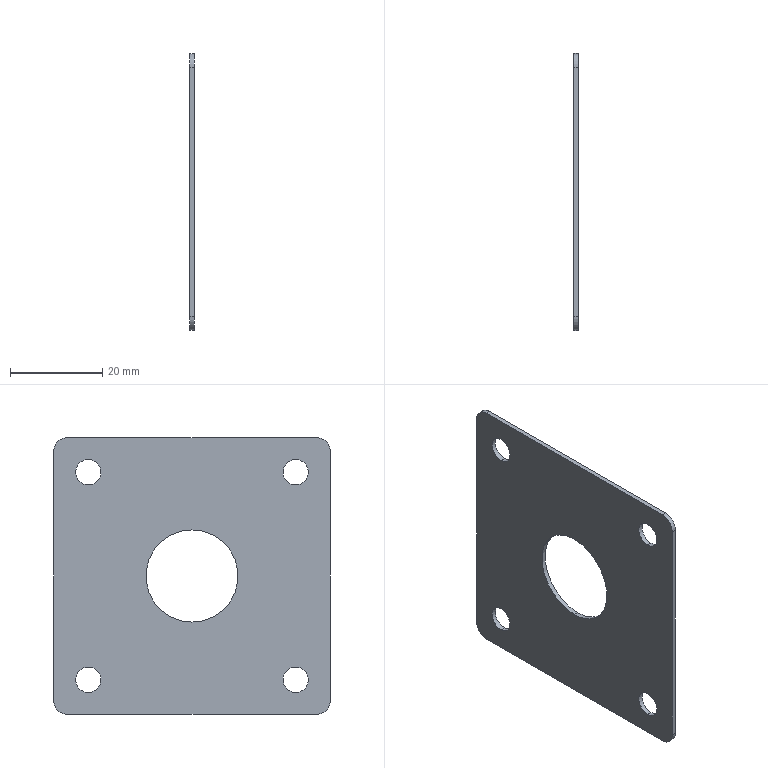Part | STEP file | FFH80-GY-022^FFH85-PL-M75-B3-01_three-axis module | 1 solid | 20 faces | box 1 x 60 x 60 mm | volume 3183 mm3 | cylinder 14 | plane 6 | commonest cylinder face diameters 5.5 x8 6 x4 20 x2
STEP:
#1=CARTESIAN_POINT('',(0.,22.5,-19.75));
#2=VERTEX_POINT('',#1);
#3=CARTESIAN_POINT('',(0.,22.5,-25.25));
#4=VERTEX_POINT('',#3);
#5=CARTESIAN_POINT('',(0.,22.5,-22.5));
#6=DIRECTION('',(1.,0.,0.));
#7=DIRECTION('',(0.,0.,-1.));
#8=AXIS2_PLACEMENT_3D('',#5,#6,#7);
#9=CIRCLE('',#8,2.75);
#10=EDGE_CURVE('',#2,#4,#9,.T.);
#11=ORIENTED_EDGE('',*,*,#10,.F.);
#12=CARTESIAN_POINT('',(1.,22.5,-19.75));
#13=VERTEX_POINT('',#12);
#14=CARTESIAN_POINT('',(1.,22.5,-19.75));
#15=DIRECTION('',(1.,0.,0.));
#16=VECTOR('',#15,1000.);
#17=LINE('',#14,#16);
#18=EDGE_CURVE('',#2,#13,#17,.T.);
#19=ORIENTED_EDGE('',*,*,#18,.T.);
#20=CARTESIAN_POINT('',(1.,22.5,-25.25));
#21=VERTEX_POINT('',#20);
#22=CARTESIAN_POINT('',(1.,22.5,-22.5));
#23=DIRECTION('',(1.,0.,0.));
#24=DIRECTION('',(0.,0.,-1.));
#25=AXIS2_PLACEMENT_3D('',#22,#23,#24);
#26=CIRCLE('',#25,2.75);
#27=EDGE_CURVE('',#13,#21,#26,.T.);
#28=ORIENTED_EDGE('',*,*,#27,.T.);
#29=CARTESIAN_POINT('',(1.,22.5,-25.25));
#30=DIRECTION('',(1.,0.,0.));
#31=VECTOR('',#30,1000.);
#32=LINE('',#29,#31);
#33=EDGE_CURVE('',#4,#21,#32,.T.);
#34=ORIENTED_EDGE('',*,*,#33,.F.);
#35=EDGE_LOOP('',(#11,#19,#28,#34));
#36=FACE_OUTER_BOUND('',#35,.T.);
#37=CARTESIAN_POINT('',(1.,22.5,-22.5));
#38=DIRECTION('',(1.,0.,0.));
#39=DIRECTION('',(0.,0.,-1.));
#40=AXIS2_PLACEMENT_3D('',#37,#38,#39);
#41=CYLINDRICAL_SURFACE('',#40,2.75);
#42=ADVANCED_FACE('',(#36),#41,.F.);
#43=CARTESIAN_POINT('',(0.,22.5,25.25));
#44=VERTEX_POINT('',#43);
#45=CARTESIAN_POINT('',(0.,22.5,19.75));
#46=VERTEX_POINT('',#45);
#47=CARTESIAN_POINT('',(0.,22.5,22.5));
#48=DIRECTION('',(1.,0.,0.));
#49=DIRECTION('',(0.,0.,-1.));
#50=AXIS2_PLACEMENT_3D('',#47,#48,#49);
#51=CIRCLE('',#50,2.75);
#52=EDGE_CURVE('',#44,#46,#51,.T.);
#53=ORIENTED_EDGE('',*,*,#52,.F.);
#54=CARTESIAN_POINT('',(1.,22.5,25.25));
#55=VERTEX_POINT('',#54);
#56=CARTESIAN_POINT('',(1.,22.5,25.25));
#57=DIRECTION('',(1.,0.,0.));
#58=VECTOR('',#57,1000.);
#59=LINE('',#56,#58);
#60=EDGE_CURVE('',#44,#55,#59,.T.);
#61=ORIENTED_EDGE('',*,*,#60,.T.);
#62=CARTESIAN_POINT('',(1.,22.5,19.75));
#63=VERTEX_POINT('',#62);
#64=CARTESIAN_POINT('',(1.,22.5,22.5));
#65=DIRECTION('',(1.,0.,0.));
#66=DIRECTION('',(0.,0.,-1.));
#67=AXIS2_PLACEMENT_3D('',#64,#65,#66);
#68=CIRCLE('',#67,2.75);
#69=EDGE_CURVE('',#55,#63,#68,.T.);
#70=ORIENTED_EDGE('',*,*,#69,.T.);
#71=CARTESIAN_POINT('',(1.,22.5,19.75));
#72=DIRECTION('',(1.,0.,0.));
#73=VECTOR('',#72,1000.);
#74=LINE('',#71,#73);
#75=EDGE_CURVE('',#46,#63,#74,.T.);
#76=ORIENTED_EDGE('',*,*,#75,.F.);
#77=EDGE_LOOP('',(#53,#61,#70,#76));
#78=FACE_OUTER_BOUND('',#77,.T.);
#79=CARTESIAN_POINT('',(1.,22.5,22.5));
#80=DIRECTION('',(1.,0.,0.));
#81=DIRECTION('',(0.,0.,-1.));
#82=AXIS2_PLACEMENT_3D('',#79,#80,#81);
#83=CYLINDRICAL_SURFACE('',#82,2.75);
#84=ADVANCED_FACE('',(#78),#83,.F.);
#85=CARTESIAN_POINT('',(0.,-22.5,-19.75));
#86=VERTEX_POINT('',#85);
#87=CARTESIAN_POINT('',(0.,-22.5,-25.25));
#88=VERTEX_POINT('',#87);
#89=CARTESIAN_POINT('',(0.,-22.5,-22.5));
#90=DIRECTION('',(1.,0.,0.));
#91=DIRECTION('',(0.,0.,-1.));
#92=AXIS2_PLACEMENT_3D('',#89,#90,#91);
#93=CIRCLE('',#92,2.75);
#94=EDGE_CURVE('',#86,#88,#93,.T.);
#95=ORIENTED_EDGE('',*,*,#94,.F.);
#96=CARTESIAN_POINT('',(1.,-22.5,-19.75));
#97=VERTEX_POINT('',#96);
#98=CARTESIAN_POINT('',(1.,-22.5,-19.75));
#99=DIRECTION('',(1.,0.,0.));
#100=VECTOR('',#99,1000.);
#101=LINE('',#98,#100);
#102=EDGE_CURVE('',#86,#97,#101,.T.);
#103=ORIENTED_EDGE('',*,*,#102,.T.);
#104=CARTESIAN_POINT('',(1.,-22.5,-25.25));
#105=VERTEX_POINT('',#104);
#106=CARTESIAN_POINT('',(1.,-22.5,-22.5));
#107=DIRECTION('',(1.,0.,0.));
#108=DIRECTION('',(0.,0.,-1.));
#109=AXIS2_PLACEMENT_3D('',#106,#107,#108);
#110=CIRCLE('',#109,2.75);
#111=EDGE_CURVE('',#97,#105,#110,.T.);
#112=ORIENTED_EDGE('',*,*,#111,.T.);
#113=CARTESIAN_POINT('',(1.,-22.5,-25.25));
#114=DIRECTION('',(1.,0.,0.));
#115=VECTOR('',#114,1000.);
#116=LINE('',#113,#115);
#117=EDGE_CURVE('',#88,#105,#116,.T.);
#118=ORIENTED_EDGE('',*,*,#117,.F.);
#119=EDGE_LOOP('',(#95,#103,#112,#118));
#120=FACE_OUTER_BOUND('',#119,.T.);
#121=CARTESIAN_POINT('',(1.,-22.5,-22.5));
#122=DIRECTION('',(1.,0.,0.));
#123=DIRECTION('',(0.,0.,-1.));
#124=AXIS2_PLACEMENT_3D('',#121,#122,#123);
#125=CYLINDRICAL_SURFACE('',#124,2.75);
#126=ADVANCED_FACE('',(#120),#125,.F.);
#127=CARTESIAN_POINT('',(0.,-22.5,25.25));
#128=VERTEX_POINT('',#127);
#129=CARTESIAN_POINT('',(0.,-22.5,19.75));
#130=VERTEX_POINT('',#129);
#131=CARTESIAN_POINT('',(0.,-22.5,22.5));
#132=DIRECTION('',(1.,0.,0.));
#133=DIRECTION('',(0.,0.,-1.));
#134=AXIS2_PLACEMENT_3D('',#131,#132,#133);
#135=CIRCLE('',#134,2.75);
#136=EDGE_CURVE('',#128,#130,#135,.T.);
#137=ORIENTED_EDGE('',*,*,#136,.F.);
#138=CARTESIAN_POINT('',(1.,-22.5,25.25));
#139=VERTEX_POINT('',#138);
#140=CARTESIAN_POINT('',(1.,-22.5,25.25));
#141=DIRECTION('',(1.,0.,0.));
#142=VECTOR('',#141,1000.);
#143=LINE('',#140,#142);
#144=EDGE_CURVE('',#128,#139,#143,.T.);
#145=ORIENTED_EDGE('',*,*,#144,.T.);
#146=CARTESIAN_POINT('',(1.,-22.5,19.75));
#147=VERTEX_POINT('',#146);
#148=CARTESIAN_POINT('',(1.,-22.5,22.5));
#149=DIRECTION('',(1.,0.,0.));
#150=DIRECTION('',(0.,0.,-1.));
#151=AXIS2_PLACEMENT_3D('',#148,#149,#150);
#152=CIRCLE('',#151,2.75);
#153=EDGE_CURVE('',#139,#147,#152,.T.);
#154=ORIENTED_EDGE('',*,*,#153,.T.);
#155=CARTESIAN_POINT('',(1.,-22.5,19.75));
#156=DIRECTION('',(1.,0.,0.));
#157=VECTOR('',#156,1000.);
#158=LINE('',#155,#157);
#159=EDGE_CURVE('',#130,#147,#158,.T.);
#160=ORIENTED_EDGE('',*,*,#159,.F.);
#161=EDGE_LOOP('',(#137,#145,#154,#160));
#162=FACE_OUTER_BOUND('',#161,.T.);
#163=CARTESIAN_POINT('',(1.,-22.5,22.5));
#164=DIRECTION('',(1.,0.,0.));
#165=DIRECTION('',(0.,0.,-1.));
#166=AXIS2_PLACEMENT_3D('',#163,#164,#165);
#167=CYLINDRICAL_SURFACE('',#166,2.75);
#168=ADVANCED_FACE('',(#162),#167,.F.);
#169=CARTESIAN_POINT('',(0.,0.,10.));
#170=VERTEX_POINT('',#169);
#171=CARTESIAN_POINT('',(0.,0.,-10.));
#172=VERTEX_POINT('',#171);
#173=CARTESIAN_POINT('',(0.,0.,0.));
#174=DIRECTION('',(1.,0.,0.));
#175=DIRECTION('',(0.,0.,-1.));
#176=AXIS2_PLACEMENT_3D('',#173,#174,#175);
#177=CIRCLE('',#176,10.);
#178=EDGE_CURVE('',#170,#172,#177,.T.);
#179=ORIENTED_EDGE('',*,*,#178,.F.);
#180=CARTESIAN_POINT('',(1.,0.,10.));
#181=VERTEX_POINT('',#180);
#182=CARTESIAN_POINT('',(0.,0.,10.));
#183=DIRECTION('',(1.,0.,0.));
#184=VECTOR('',#183,1000.);
#185=LINE('',#182,#184);
#186=EDGE_CURVE('',#170,#181,#185,.T.);
#187=ORIENTED_EDGE('',*,*,#186,.T.);
#188=CARTESIAN_POINT('',(1.,0.,-10.));
#189=VERTEX_POINT('',#188);
#190=CARTESIAN_POINT('',(1.,0.,0.));
#191=DIRECTION('',(1.,0.,0.));
#192=DIRECTION('',(0.,0.,-1.));
#193=AXIS2_PLACEMENT_3D('',#190,#191,#192);
#194=CIRCLE('',#193,10.);
#195=EDGE_CURVE('',#181,#189,#194,.T.);
#196=ORIENTED_EDGE('',*,*,#195,.T.);
#197=CARTESIAN_POINT('',(0.,0.,-10.));
#198=DIRECTION('',(1.,0.,0.));
#199=VECTOR('',#198,1000.);
#200=LINE('',#197,#199);
#201=EDGE_CURVE('',#172,#189,#200,.T.);
#202=ORIENTED_EDGE('',*,*,#201,.F.);
#203=EDGE_LOOP('',(#179,#187,#196,#202));
#204=FACE_OUTER_BOUND('',#203,.T.);
#205=CARTESIAN_POINT('',(0.,0.,0.));
#206=DIRECTION('',(1.,0.,0.));
#207=DIRECTION('',(0.,0.,-1.));
#208=AXIS2_PLACEMENT_3D('',#205,#206,#207);
#209=CYLINDRICAL_SURFACE('',#208,10.);
#210=ADVANCED_FACE('',(#204),#209,.F.);
#211=CARTESIAN_POINT('',(1.,22.5,-22.5));
#212=DIRECTION('',(1.,0.,0.));
#213=DIRECTION('',(0.,0.,-1.));
#214=AXIS2_PLACEMENT_3D('',#211,#212,#213);
#215=CIRCLE('',#214,2.75);
#216=EDGE_CURVE('',#21,#13,#215,.T.);
#217=ORIENTED_EDGE('',*,*,#216,.F.);
#218=ORIENTED_EDGE('',*,*,#27,.F.);
#219=EDGE_LOOP('',(#217,#218));
#220=FACE_BOUND('',#219,.T.);
#221=CARTESIAN_POINT('',(1.,22.5,22.5));
#222=DIRECTION('',(1.,0.,0.));
#223=DIRECTION('',(0.,0.,-1.));
#224=AXIS2_PLACEMENT_3D('',#221,#222,#223);
#225=CIRCLE('',#224,2.75);
#226=EDGE_CURVE('',#63,#55,#225,.T.);
#227=ORIENTED_EDGE('',*,*,#226,.F.);
#228=ORIENTED_EDGE('',*,*,#69,.F.);
#229=EDGE_LOOP('',(#227,#228));
#230=FACE_BOUND('',#229,.T.);
#231=CARTESIAN_POINT('',(1.,-22.5,-22.5));
#232=DIRECTION('',(1.,0.,0.));
#233=DIRECTION('',(0.,0.,-1.));
#234=AXIS2_PLACEMENT_3D('',#231,#232,#233);
#235=CIRCLE('',#234,2.75);
#236=EDGE_CURVE('',#105,#97,#235,.T.);
#237=ORIENTED_EDGE('',*,*,#236,.F.);
#238=ORIENTED_EDGE('',*,*,#111,.F.);
#239=EDGE_LOOP('',(#237,#238));
#240=FACE_BOUND('',#239,.T.);
#241=CARTESIAN_POINT('',(1.,-22.5,22.5));
#242=DIRECTION('',(1.,0.,0.));
#243=DIRECTION('',(0.,0.,-1.));
#244=AXIS2_PLACEMENT_3D('',#241,#242,#243);
#245=CIRCLE('',#244,2.75);
#246=EDGE_CURVE('',#147,#139,#245,.T.);
#247=ORIENTED_EDGE('',*,*,#246,.F.);
#248=ORIENTED_EDGE('',*,*,#153,.F.);
#249=EDGE_LOOP('',(#247,#248));
#250=FACE_BOUND('',#249,.T.);
#251=CARTESIAN_POINT('',(1.,-30.,-27.));
#252=VERTEX_POINT('',#251);
#253=CARTESIAN_POINT('',(1.,-30.,27.));
#254=VERTEX_POINT('',#253);
#255=CARTESIAN_POINT('',(1.,-30.,0.));
#256=DIRECTION('',(0.,0.,1.));
#257=VECTOR('',#256,1000.);
#258=LINE('',#255,#257);
#259=EDGE_CURVE('',#252,#254,#258,.T.);
#260=ORIENTED_EDGE('',*,*,#259,.F.);
#261=CARTESIAN_POINT('',(1.,-27.,-30.));
#262=VERTEX_POINT('',#261);
#263=CARTESIAN_POINT('',(1.,-27.,-27.));
#264=DIRECTION('',(-1.,0.,0.));
#265=DIRECTION('',(0.,0.,1.));
#266=AXIS2_PLACEMENT_3D('',#263,#264,#265);
#267=CIRCLE('',#266,3.);
#268=EDGE_CURVE('',#262,#252,#267,.T.);
#269=ORIENTED_EDGE('',*,*,#268,.F.);
#270=CARTESIAN_POINT('',(1.,27.,-30.));
#271=VERTEX_POINT('',#270);
#272=CARTESIAN_POINT('',(1.,0.,-30.));
#273=DIRECTION('',(0.,-1.,0.));
#274=VECTOR('',#273,1000.);
#275=LINE('',#272,#274);
#276=EDGE_CURVE('',#271,#262,#275,.T.);
#277=ORIENTED_EDGE('',*,*,#276,.F.);
#278=CARTESIAN_POINT('',(1.,30.,-27.));
#279=VERTEX_POINT('',#278);
#280=CARTESIAN_POINT('',(1.,27.,-27.));
#281=DIRECTION('',(-1.,0.,0.));
#282=DIRECTION('',(0.,0.,1.));
#283=AXIS2_PLACEMENT_3D('',#280,#281,#282);
#284=CIRCLE('',#283,3.);
#285=EDGE_CURVE('',#279,#271,#284,.T.);
#286=ORIENTED_EDGE('',*,*,#285,.F.);
#287=CARTESIAN_POINT('',(1.,30.,27.));
#288=VERTEX_POINT('',#287);
#289=CARTESIAN_POINT('',(1.,30.,0.));
#290=DIRECTION('',(0.,0.,-1.));
#291=VECTOR('',#290,1000.);
#292=LINE('',#289,#291);
#293=EDGE_CURVE('',#288,#279,#292,.T.);
#294=ORIENTED_EDGE('',*,*,#293,.F.);
#295=CARTESIAN_POINT('',(1.,27.,30.));
#296=VERTEX_POINT('',#295);
#297=CARTESIAN_POINT('',(1.,27.,27.));
#298=DIRECTION('',(-1.,0.,0.));
#299=DIRECTION('',(0.,0.,1.));
#300=AXIS2_PLACEMENT_3D('',#297,#298,#299);
#301=CIRCLE('',#300,3.);
#302=EDGE_CURVE('',#296,#288,#301,.T.);
#303=ORIENTED_EDGE('',*,*,#302,.F.);
#304=CARTESIAN_POINT('',(1.,-27.,30.));
#305=VERTEX_POINT('',#304);
#306=CARTESIAN_POINT('',(1.,0.,30.));
#307=DIRECTION('',(0.,1.,0.));
#308=VECTOR('',#307,1000.);
#309=LINE('',#306,#308);
#310=EDGE_CURVE('',#305,#296,#309,.T.);
#311=ORIENTED_EDGE('',*,*,#310,.F.);
#312=CARTESIAN_POINT('',(1.,-27.,27.));
#313=DIRECTION('',(-1.,0.,0.));
#314=DIRECTION('',(0.,0.,1.));
#315=AXIS2_PLACEMENT_3D('',#312,#313,#314);
#316=CIRCLE('',#315,3.);
#317=EDGE_CURVE('',#254,#305,#316,.T.);
#318=ORIENTED_EDGE('',*,*,#317,.F.);
#319=EDGE_LOOP('',(#260,#269,#277,#286,#294,#303,#311,#318));
#320=FACE_OUTER_BOUND('',#319,.T.);
#321=CARTESIAN_POINT('',(1.,0.,0.));
#322=DIRECTION('',(1.,0.,0.));
#323=DIRECTION('',(0.,0.,-1.));
#324=AXIS2_PLACEMENT_3D('',#321,#322,#323);
#325=CIRCLE('',#324,10.);
#326=EDGE_CURVE('',#189,#181,#325,.T.);
#327=ORIENTED_EDGE('',*,*,#326,.F.);
#328=ORIENTED_EDGE('',*,*,#195,.F.);
#329=EDGE_LOOP('',(#327,#328));
#330=FACE_BOUND('',#329,.T.);
#331=CARTESIAN_POINT('',(1.,0.,0.));
#332=DIRECTION('',(-1.,0.,0.));
#333=DIRECTION('',(0.,0.,1.));
#334=AXIS2_PLACEMENT_3D('',#331,#332,#333);
#335=PLANE('',#334);
#336=ADVANCED_FACE('',(#220,#230,#240,#250,#320,#330),#335,.F.);
#337=ORIENTED_EDGE('',*,*,#18,.F.);
#338=CARTESIAN_POINT('',(0.,22.5,-22.5));
#339=DIRECTION('',(1.,0.,0.));
#340=DIRECTION('',(0.,0.,-1.));
#341=AXIS2_PLACEMENT_3D('',#338,#339,#340);
#342=CIRCLE('',#341,2.75);
#343=EDGE_CURVE('',#4,#2,#342,.T.);
#344=ORIENTED_EDGE('',*,*,#343,.F.);
#345=ORIENTED_EDGE('',*,*,#33,.T.);
#346=ORIENTED_EDGE('',*,*,#216,.T.);
#347=EDGE_LOOP('',(#337,#344,#345,#346));
#348=FACE_OUTER_BOUND('',#347,.T.);
#349=CARTESIAN_POINT('',(1.,22.5,-22.5));
#350=DIRECTION('',(1.,0.,0.));
#351=DIRECTION('',(0.,0.,-1.));
#352=AXIS2_PLACEMENT_3D('',#349,#350,#351);
#353=CYLINDRICAL_SURFACE('',#352,2.75);
#354=ADVANCED_FACE('',(#348),#353,.F.);
#355=ORIENTED_EDGE('',*,*,#60,.F.);
#356=CARTESIAN_POINT('',(0.,22.5,22.5));
#357=DIRECTION('',(1.,0.,0.));
#358=DIRECTION('',(0.,0.,-1.));
#359=AXIS2_PLACEMENT_3D('',#356,#357,#358);
#360=CIRCLE('',#359,2.75);
#361=EDGE_CURVE('',#46,#44,#360,.T.);
#362=ORIENTED_EDGE('',*,*,#361,.F.);
#363=ORIENTED_EDGE('',*,*,#75,.T.);
#364=ORIENTED_EDGE('',*,*,#226,.T.);
#365=EDGE_LOOP('',(#355,#362,#363,#364));
#366=FACE_OUTER_BOUND('',#365,.T.);
#367=CARTESIAN_POINT('',(1.,22.5,22.5));
#368=DIRECTION('',(1.,0.,0.));
#369=DIRECTION('',(0.,0.,-1.));
#370=AXIS2_PLACEMENT_3D('',#367,#368,#369);
#371=CYLINDRICAL_SURFACE('',#370,2.75);
#372=ADVANCED_FACE('',(#366),#371,.F.);
#373=ORIENTED_EDGE('',*,*,#102,.F.);
#374=CARTESIAN_POINT('',(0.,-22.5,-22.5));
#375=DIRECTION('',(1.,0.,0.));
#376=DIRECTION('',(0.,0.,-1.));
#377=AXIS2_PLACEMENT_3D('',#374,#375,#376);
#378=CIRCLE('',#377,2.75);
#379=EDGE_CURVE('',#88,#86,#378,.T.);
#380=ORIENTED_EDGE('',*,*,#379,.F.);
#381=ORIENTED_EDGE('',*,*,#117,.T.);
#382=ORIENTED_EDGE('',*,*,#236,.T.);
#383=EDGE_LOOP('',(#373,#380,#381,#382));
#384=FACE_OUTER_BOUND('',#383,.T.);
#385=CARTESIAN_POINT('',(1.,-22.5,-22.5));
#386=DIRECTION('',(1.,0.,0.));
#387=DIRECTION('',(0.,0.,-1.));
#388=AXIS2_PLACEMENT_3D('',#385,#386,#387);
#389=CYLINDRICAL_SURFACE('',#388,2.75);
#390=ADVANCED_FACE('',(#384),#389,.F.);
#391=ORIENTED_EDGE('',*,*,#144,.F.);
#392=CARTESIAN_POINT('',(0.,-22.5,22.5));
#393=DIRECTION('',(1.,0.,0.));
#394=DIRECTION('',(0.,0.,-1.));
#395=AXIS2_PLACEMENT_3D('',#392,#393,#394);
#396=CIRCLE('',#395,2.75);
#397=EDGE_CURVE('',#130,#128,#396,.T.);
#398=ORIENTED_EDGE('',*,*,#397,.F.);
#399=ORIENTED_EDGE('',*,*,#159,.T.);
#400=ORIENTED_EDGE('',*,*,#246,.T.);
#401=EDGE_LOOP('',(#391,#398,#399,#400));
#402=FACE_OUTER_BOUND('',#401,.T.);
#403=CARTESIAN_POINT('',(1.,-22.5,22.5));
#404=DIRECTION('',(1.,0.,0.));
#405=DIRECTION('',(0.,0.,-1.));
#406=AXIS2_PLACEMENT_3D('',#403,#404,#405);
#407=CYLINDRICAL_SURFACE('',#406,2.75);
#408=ADVANCED_FACE('',(#402),#407,.F.);
#409=ORIENTED_EDGE('',*,*,#317,.T.);
#410=CARTESIAN_POINT('',(0.,-27.,30.));
#411=VERTEX_POINT('',#410);
#412=CARTESIAN_POINT('',(1.,-27.,30.));
#413=DIRECTION('',(-1.,0.,0.));
#414=VECTOR('',#413,1000.);
#415=LINE('',#412,#414);
#416=EDGE_CURVE('',#305,#411,#415,.T.);
#417=ORIENTED_EDGE('',*,*,#416,.T.);
#418=CARTESIAN_POINT('',(0.,-30.,27.));
#419=VERTEX_POINT('',#418);
#420=CARTESIAN_POINT('',(0.,-27.,27.));
#421=DIRECTION('',(1.,0.,0.));
#422=DIRECTION('',(0.,0.,1.));
#423=AXIS2_PLACEMENT_3D('',#420,#421,#422);
#424=CIRCLE('',#423,3.);
#425=EDGE_CURVE('',#411,#419,#424,.T.);
#426=ORIENTED_EDGE('',*,*,#425,.T.);
#427=CARTESIAN_POINT('',(1.,-30.,27.));
#428=DIRECTION('',(1.,0.,0.));
#429=VECTOR('',#428,1000.);
#430=LINE('',#427,#429);
#431=EDGE_CURVE('',#419,#254,#430,.T.);
#432=ORIENTED_EDGE('',*,*,#431,.T.);
#433=EDGE_LOOP('',(#409,#417,#426,#432));
#434=FACE_OUTER_BOUND('',#433,.T.);
#435=CARTESIAN_POINT('',(1.,-27.,27.));
#436=DIRECTION('',(-1.,0.,0.));
#437=DIRECTION('',(0.,0.,1.));
#438=AXIS2_PLACEMENT_3D('',#435,#436,#437);
#439=CYLINDRICAL_SURFACE('',#438,3.);
#440=ADVANCED_FACE('',(#434),#439,.T.);
#441=CARTESIAN_POINT('',(0.,-30.,-27.));
#442=VERTEX_POINT('',#441);
#443=CARTESIAN_POINT('',(0.,-30.,-30.));
#444=DIRECTION('',(0.,0.,1.));
#445=VECTOR('',#444,1000.);
#446=LINE('',#443,#445);
#447=EDGE_CURVE('',#442,#419,#446,.T.);
#448=ORIENTED_EDGE('',*,*,#447,.F.);
#449=CARTESIAN_POINT('',(1.,-30.,-27.));
#450=DIRECTION('',(-1.,0.,0.));
#451=VECTOR('',#450,1000.);
#452=LINE('',#449,#451);
#453=EDGE_CURVE('',#252,#442,#452,.T.);
#454=ORIENTED_EDGE('',*,*,#453,.F.);
#455=ORIENTED_EDGE('',*,*,#259,.T.);
#456=ORIENTED_EDGE('',*,*,#431,.F.);
#457=EDGE_LOOP('',(#448,#454,#455,#456));
#458=FACE_OUTER_BOUND('',#457,.T.);
#459=CARTESIAN_POINT('',(1.,-30.,-30.));
#460=DIRECTION('',(0.,1.,0.));
#461=DIRECTION('',(0.,0.,1.));
#462=AXIS2_PLACEMENT_3D('',#459,#460,#461);
#463=PLANE('',#462);
#464=ADVANCED_FACE('',(#458),#463,.F.);
#465=ORIENTED_EDGE('',*,*,#268,.T.);
#466=ORIENTED_EDGE('',*,*,#453,.T.);
#467=CARTESIAN_POINT('',(0.,-27.,-30.));
#468=VERTEX_POINT('',#467);
#469=CARTESIAN_POINT('',(0.,-27.,-27.));
#470=DIRECTION('',(1.,0.,0.));
#471=DIRECTION('',(0.,0.,1.));
#472=AXIS2_PLACEMENT_3D('',#469,#470,#471);
#473=CIRCLE('',#472,3.);
#474=EDGE_CURVE('',#442,#468,#473,.T.);
#475=ORIENTED_EDGE('',*,*,#474,.T.);
#476=CARTESIAN_POINT('',(1.,-27.,-30.));
#477=DIRECTION('',(1.,0.,0.));
#478=VECTOR('',#477,1000.);
#479=LINE('',#476,#478);
#480=EDGE_CURVE('',#468,#262,#479,.T.);
#481=ORIENTED_EDGE('',*,*,#480,.T.);
#482=EDGE_LOOP('',(#465,#466,#475,#481));
#483=FACE_OUTER_BOUND('',#482,.T.);
#484=CARTESIAN_POINT('',(1.,-27.,-27.));
#485=DIRECTION('',(-1.,0.,0.));
#486=DIRECTION('',(0.,0.,1.));
#487=AXIS2_PLACEMENT_3D('',#484,#485,#486);
#488=CYLINDRICAL_SURFACE('',#487,3.);
#489=ADVANCED_FACE('',(#483),#488,.T.);
#490=CARTESIAN_POINT('',(0.,27.,-30.));
#491=VERTEX_POINT('',#490);
#492=CARTESIAN_POINT('',(0.,30.,-30.));
#493=DIRECTION('',(0.,-1.,0.));
#494=VECTOR('',#493,1000.);
#495=LINE('',#492,#494);
#496=EDGE_CURVE('',#491,#468,#495,.T.);
#497=ORIENTED_EDGE('',*,*,#496,.F.);
#498=CARTESIAN_POINT('',(1.,27.,-30.));
#499=DIRECTION('',(-1.,0.,0.));
#500=VECTOR('',#499,1000.);
#501=LINE('',#498,#500);
#502=EDGE_CURVE('',#271,#491,#501,.T.);
#503=ORIENTED_EDGE('',*,*,#502,.F.);
#504=ORIENTED_EDGE('',*,*,#276,.T.);
#505=ORIENTED_EDGE('',*,*,#480,.F.);
#506=EDGE_LOOP('',(#497,#503,#504,#505));
#507=FACE_OUTER_BOUND('',#506,.T.);
#508=CARTESIAN_POINT('',(1.,30.,-30.));
#509=DIRECTION('',(0.,0.,1.));
#510=DIRECTION('',(0.,-1.,0.));
#511=AXIS2_PLACEMENT_3D('',#508,#509,#510);
#512=PLANE('',#511);
#513=ADVANCED_FACE('',(#507),#512,.F.);
#514=ORIENTED_EDGE('',*,*,#285,.T.);
#515=ORIENTED_EDGE('',*,*,#502,.T.);
#516=CARTESIAN_POINT('',(0.,30.,-27.));
#517=VERTEX_POINT('',#516);
#518=CARTESIAN_POINT('',(0.,27.,-27.));
#519=DIRECTION('',(1.,0.,0.));
#520=DIRECTION('',(0.,0.,1.));
#521=AXIS2_PLACEMENT_3D('',#518,#519,#520);
#522=CIRCLE('',#521,3.);
#523=EDGE_CURVE('',#491,#517,#522,.T.);
#524=ORIENTED_EDGE('',*,*,#523,.T.);
#525=CARTESIAN_POINT('',(1.,30.,-27.));
#526=DIRECTION('',(1.,0.,0.));
#527=VECTOR('',#526,1000.);
#528=LINE('',#525,#527);
#529=EDGE_CURVE('',#517,#279,#528,.T.);
#530=ORIENTED_EDGE('',*,*,#529,.T.);
#531=EDGE_LOOP('',(#514,#515,#524,#530));
#532=FACE_OUTER_BOUND('',#531,.T.);
#533=CARTESIAN_POINT('',(1.,27.,-27.));
#534=DIRECTION('',(-1.,0.,0.));
#535=DIRECTION('',(0.,0.,1.));
#536=AXIS2_PLACEMENT_3D('',#533,#534,#535);
#537=CYLINDRICAL_SURFACE('',#536,3.);
#538=ADVANCED_FACE('',(#532),#537,.T.);
#539=CARTESIAN_POINT('',(0.,30.,27.));
#540=VERTEX_POINT('',#539);
#541=CARTESIAN_POINT('',(0.,30.,-30.));
#542=DIRECTION('',(0.,0.,-1.));
#543=VECTOR('',#542,1000.);
#544=LINE('',#541,#543);
#545=EDGE_CURVE('',#540,#517,#544,.T.);
#546=ORIENTED_EDGE('',*,*,#545,.F.);
#547=CARTESIAN_POINT('',(1.,30.,27.));
#548=DIRECTION('',(-1.,0.,0.));
#549=VECTOR('',#548,1000.);
#550=LINE('',#547,#549);
#551=EDGE_CURVE('',#288,#540,#550,.T.);
#552=ORIENTED_EDGE('',*,*,#551,.F.);
#553=ORIENTED_EDGE('',*,*,#293,.T.);
#554=ORIENTED_EDGE('',*,*,#529,.F.);
#555=EDGE_LOOP('',(#546,#552,#553,#554));
#556=FACE_OUTER_BOUND('',#555,.T.);
#557=CARTESIAN_POINT('',(1.,30.,-30.));
#558=DIRECTION('',(0.,-1.,0.));
#559=DIRECTION('',(0.,0.,-1.));
#560=AXIS2_PLACEMENT_3D('',#557,#558,#559);
#561=PLANE('',#560);
#562=ADVANCED_FACE('',(#556),#561,.F.);
#563=ORIENTED_EDGE('',*,*,#302,.T.);
#564=ORIENTED_EDGE('',*,*,#551,.T.);
#565=CARTESIAN_POINT('',(0.,27.,30.));
#566=VERTEX_POINT('',#565);
#567=CARTESIAN_POINT('',(0.,27.,27.));
#568=DIRECTION('',(1.,0.,0.));
#569=DIRECTION('',(0.,0.,1.));
#570=AXIS2_PLACEMENT_3D('',#567,#568,#569);
#571=CIRCLE('',#570,3.);
#572=EDGE_CURVE('',#540,#566,#571,.T.);
#573=ORIENTED_EDGE('',*,*,#572,.T.);
#574=CARTESIAN_POINT('',(1.,27.,30.));
#575=DIRECTION('',(1.,0.,0.));
#576=VECTOR('',#575,1000.);
#577=LINE('',#574,#576);
#578=EDGE_CURVE('',#566,#296,#577,.T.);
#579=ORIENTED_EDGE('',*,*,#578,.T.);
#580=EDGE_LOOP('',(#563,#564,#573,#579));
#581=FACE_OUTER_BOUND('',#580,.T.);
#582=CARTESIAN_POINT('',(1.,27.,27.));
#583=DIRECTION('',(-1.,0.,0.));
#584=DIRECTION('',(0.,0.,1.));
#585=AXIS2_PLACEMENT_3D('',#582,#583,#584);
#586=CYLINDRICAL_SURFACE('',#585,3.);
#587=ADVANCED_FACE('',(#581),#586,.T.);
#588=ORIENTED_EDGE('',*,*,#310,.T.);
#589=ORIENTED_EDGE('',*,*,#578,.F.);
#590=CARTESIAN_POINT('',(0.,30.,30.));
#591=DIRECTION('',(0.,1.,0.));
#592=VECTOR('',#591,1000.);
#593=LINE('',#590,#592);
#594=EDGE_CURVE('',#411,#566,#593,.T.);
#595=ORIENTED_EDGE('',*,*,#594,.F.);
#596=ORIENTED_EDGE('',*,*,#416,.F.);
#597=EDGE_LOOP('',(#588,#589,#595,#596));
#598=FACE_OUTER_BOUND('',#597,.T.);
#599=CARTESIAN_POINT('',(1.,30.,30.));
#600=DIRECTION('',(0.,0.,-1.));
#601=DIRECTION('',(0.,1.,0.));
#602=AXIS2_PLACEMENT_3D('',#599,#600,#601);
#603=PLANE('',#602);
#604=ADVANCED_FACE('',(#598),#603,.F.);
#605=ORIENTED_EDGE('',*,*,#186,.F.);
#606=CARTESIAN_POINT('',(0.,0.,0.));
#607=DIRECTION('',(1.,0.,0.));
#608=DIRECTION('',(0.,0.,-1.));
#609=AXIS2_PLACEMENT_3D('',#606,#607,#608);
#610=CIRCLE('',#609,10.);
#611=EDGE_CURVE('',#172,#170,#610,.T.);
#612=ORIENTED_EDGE('',*,*,#611,.F.);
#613=ORIENTED_EDGE('',*,*,#201,.T.);
#614=ORIENTED_EDGE('',*,*,#326,.T.);
#615=EDGE_LOOP('',(#605,#612,#613,#614));
#616=FACE_OUTER_BOUND('',#615,.T.);
#617=CARTESIAN_POINT('',(0.,0.,0.));
#618=DIRECTION('',(1.,0.,0.));
#619=DIRECTION('',(0.,0.,-1.));
#620=AXIS2_PLACEMENT_3D('',#617,#618,#619);
#621=CYLINDRICAL_SURFACE('',#620,10.);
#622=ADVANCED_FACE('',(#616),#621,.F.);
#623=ORIENTED_EDGE('',*,*,#343,.T.);
#624=ORIENTED_EDGE('',*,*,#10,.T.);
#625=EDGE_LOOP('',(#623,#624));
#626=FACE_BOUND('',#625,.T.);
#627=ORIENTED_EDGE('',*,*,#361,.T.);
#628=ORIENTED_EDGE('',*,*,#52,.T.);
#629=EDGE_LOOP('',(#627,#628));
#630=FACE_BOUND('',#629,.T.);
#631=ORIENTED_EDGE('',*,*,#379,.T.);
#632=ORIENTED_EDGE('',*,*,#94,.T.);
#633=EDGE_LOOP('',(#631,#632));
#634=FACE_BOUND('',#633,.T.);
#635=ORIENTED_EDGE('',*,*,#397,.T.);
#636=ORIENTED_EDGE('',*,*,#136,.T.);
#637=EDGE_LOOP('',(#635,#636));
#638=FACE_BOUND('',#637,.T.);
#639=ORIENTED_EDGE('',*,*,#545,.T.);
#640=ORIENTED_EDGE('',*,*,#523,.F.);
#641=ORIENTED_EDGE('',*,*,#496,.T.);
#642=ORIENTED_EDGE('',*,*,#474,.F.);
#643=ORIENTED_EDGE('',*,*,#447,.T.);
#644=ORIENTED_EDGE('',*,*,#425,.F.);
#645=ORIENTED_EDGE('',*,*,#594,.T.);
#646=ORIENTED_EDGE('',*,*,#572,.F.);
#647=EDGE_LOOP('',(#639,#640,#641,#642,#643,#644,#645,#646));
#648=FACE_OUTER_BOUND('',#647,.T.);
#649=ORIENTED_EDGE('',*,*,#611,.T.);
#650=ORIENTED_EDGE('',*,*,#178,.T.);
#651=EDGE_LOOP('',(#649,#650));
#652=FACE_BOUND('',#651,.T.);
#653=CARTESIAN_POINT('',(0.,0.,0.));
#654=DIRECTION('',(-1.,0.,0.));
#655=DIRECTION('',(0.,0.,1.));
#656=AXIS2_PLACEMENT_3D('',#653,#654,#655);
#657=PLANE('',#656);
#658=ADVANCED_FACE('',(#626,#630,#634,#638,#648,#652),#657,.T.);
#659=CLOSED_SHELL('',(#42,#84,#126,#168,#210,#336,#354,#372,#390,#408,#440,#464,#489,#513,#538,#562,#587,#604,#622,#658));
#660=MANIFOLD_SOLID_BREP('',#659);
#661=CARTESIAN_POINT('',(0.,0.,0.));
#662=DIRECTION('',(0.,0.,1.));
#663=DIRECTION('',(1.,0.,0.));
#664=AXIS2_PLACEMENT_3D('',#661,#662,#663);
#665=(LENGTH_UNIT()NAMED_UNIT(*)SI_UNIT(.MILLI.,.METRE.));
#666=UNCERTAINTY_MEASURE_WITH_UNIT(LENGTH_MEASURE(0.00001),#665,'','');
#667=(NAMED_UNIT(*)PLANE_ANGLE_UNIT()SI_UNIT($,.RADIAN.));
#668=(NAMED_UNIT(*)SI_UNIT($,.STERADIAN.)SOLID_ANGLE_UNIT());
#669=(GEOMETRIC_REPRESENTATION_CONTEXT(3)GLOBAL_UNCERTAINTY_ASSIGNED_CONTEXT((#666))GLOBAL_UNIT_ASSIGNED_CONTEXT((#665,#667,#668))REPRESENTATION_CONTEXT('',''));
#670=ADVANCED_BREP_SHAPE_REPRESENTATION('',(#660,#664),#669);